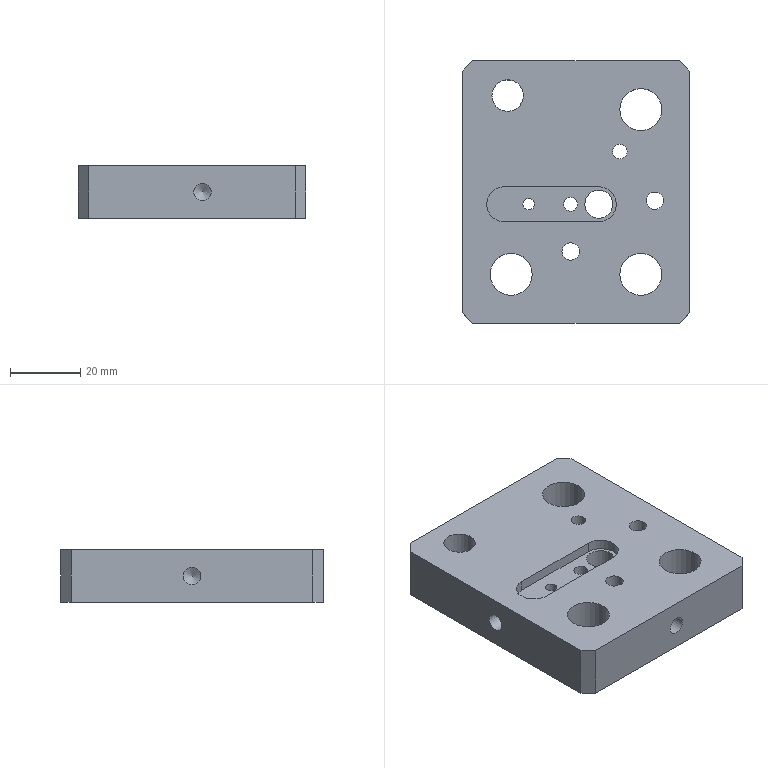Part | NX | features BREP 1 | 1 solid | 29 faces | box 65 x 75 x 15 mm | volume 63504 mm3 | cylinder 14 | plane 13 | cone 2 | commonest cylinder face diameters 5 x4 12 x3 10 x2 3.3 x1 4 x1 4.2 x1
STEP:
#1=CARTESIAN_POINT('',(32.5,-34.5,0.));
#2=VERTEX_POINT('',#1);
#3=CARTESIAN_POINT('',(32.5,34.5,0.));
#4=VERTEX_POINT('',#3);
#5=CARTESIAN_POINT('',(32.5,37.5,0.));
#6=DIRECTION('',(0.,1.,0.));
#7=VECTOR('',#6,1000.);
#8=LINE('',#5,#7);
#9=EDGE_CURVE('',#2,#4,#8,.T.);
#10=ORIENTED_EDGE('',*,*,#9,.F.);
#11=CARTESIAN_POINT('',(32.5,-34.5,-15.));
#12=VERTEX_POINT('',#11);
#13=CARTESIAN_POINT('',(32.5,-34.5,-15.));
#14=DIRECTION('',(0.,0.,1.));
#15=VECTOR('',#14,1000.);
#16=LINE('',#13,#15);
#17=EDGE_CURVE('',#12,#2,#16,.T.);
#18=ORIENTED_EDGE('',*,*,#17,.F.);
#19=CARTESIAN_POINT('',(32.5,34.5,-15.));
#20=VERTEX_POINT('',#19);
#21=CARTESIAN_POINT('',(32.5,37.5,-15.));
#22=DIRECTION('',(0.,1.,0.));
#23=VECTOR('',#22,1000.);
#24=LINE('',#21,#23);
#25=EDGE_CURVE('',#12,#20,#24,.T.);
#26=ORIENTED_EDGE('',*,*,#25,.T.);
#27=CARTESIAN_POINT('',(32.5,34.5,-15.));
#28=DIRECTION('',(0.,0.,-1.));
#29=VECTOR('',#28,1000.);
#30=LINE('',#27,#29);
#31=EDGE_CURVE('',#4,#20,#30,.T.);
#32=ORIENTED_EDGE('',*,*,#31,.F.);
#33=EDGE_LOOP('',(#10,#18,#26,#32));
#34=FACE_BOUND('',#33,.T.);
#35=CARTESIAN_POINT('',(32.5,37.5,-15.));
#36=DIRECTION('',(-1.,0.,0.));
#37=DIRECTION('',(0.,1.,0.));
#38=AXIS2_PLACEMENT_3D('',#35,#36,#37);
#39=PLANE('',#38);
#40=ADVANCED_FACE('',(#34),#39,.F.);
#41=CARTESIAN_POINT('',(29.5,37.5,-15.));
#42=VERTEX_POINT('',#41);
#43=CARTESIAN_POINT('',(-29.5,37.5,-15.));
#44=VERTEX_POINT('',#43);
#45=CARTESIAN_POINT('',(-32.5,37.5,-15.));
#46=DIRECTION('',(-1.,0.,0.));
#47=VECTOR('',#46,1000.);
#48=LINE('',#45,#47);
#49=EDGE_CURVE('',#42,#44,#48,.T.);
#50=ORIENTED_EDGE('',*,*,#49,.T.);
#51=CARTESIAN_POINT('',(-29.5,37.5,0.));
#52=VERTEX_POINT('',#51);
#53=CARTESIAN_POINT('',(-29.5,37.5,-15.));
#54=DIRECTION('',(0.,0.,-1.));
#55=VECTOR('',#54,1000.);
#56=LINE('',#53,#55);
#57=EDGE_CURVE('',#52,#44,#56,.T.);
#58=ORIENTED_EDGE('',*,*,#57,.F.);
#59=CARTESIAN_POINT('',(29.5,37.5,0.));
#60=VERTEX_POINT('',#59);
#61=CARTESIAN_POINT('',(-32.5,37.5,0.));
#62=DIRECTION('',(-1.,0.,0.));
#63=VECTOR('',#62,1000.);
#64=LINE('',#61,#63);
#65=EDGE_CURVE('',#60,#52,#64,.T.);
#66=ORIENTED_EDGE('',*,*,#65,.F.);
#67=CARTESIAN_POINT('',(29.5,37.5,-15.));
#68=DIRECTION('',(0.,0.,1.));
#69=VECTOR('',#68,1000.);
#70=LINE('',#67,#69);
#71=EDGE_CURVE('',#42,#60,#70,.T.);
#72=ORIENTED_EDGE('',*,*,#71,.F.);
#73=EDGE_LOOP('',(#50,#58,#66,#72));
#74=FACE_BOUND('',#73,.T.);
#75=CARTESIAN_POINT('',(-32.5,37.5,-15.));
#76=DIRECTION('',(0.,-1.,0.));
#77=DIRECTION('',(0.,0.,-1.));
#78=AXIS2_PLACEMENT_3D('',#75,#76,#77);
#79=PLANE('',#78);
#80=ADVANCED_FACE('',(#74),#79,.F.);
#81=CARTESIAN_POINT('',(-32.5,0.,-10.));
#82=VERTEX_POINT('',#81);
#83=CARTESIAN_POINT('',(-32.5,0.,-7.5));
#84=DIRECTION('',(1.,0.,0.));
#85=DIRECTION('',(0.,0.,-1.));
#86=AXIS2_PLACEMENT_3D('',#83,#84,#85);
#87=CIRCLE('',#86,2.5);
#88=EDGE_CURVE('',#82,#82,#87,.T.);
#89=ORIENTED_EDGE('',*,*,#88,.T.);
#90=EDGE_LOOP('',(#89));
#91=FACE_BOUND('',#90,.T.);
#92=CARTESIAN_POINT('',(-32.5,34.5,-15.));
#93=VERTEX_POINT('',#92);
#94=CARTESIAN_POINT('',(-32.5,-34.5,-15.));
#95=VERTEX_POINT('',#94);
#96=CARTESIAN_POINT('',(-32.5,37.5,-15.));
#97=DIRECTION('',(0.,-1.,0.));
#98=VECTOR('',#97,1000.);
#99=LINE('',#96,#98);
#100=EDGE_CURVE('',#93,#95,#99,.T.);
#101=ORIENTED_EDGE('',*,*,#100,.T.);
#102=CARTESIAN_POINT('',(-32.5,-34.5,0.));
#103=VERTEX_POINT('',#102);
#104=CARTESIAN_POINT('',(-32.5,-34.5,-15.));
#105=DIRECTION('',(0.,0.,-1.));
#106=VECTOR('',#105,1000.);
#107=LINE('',#104,#106);
#108=EDGE_CURVE('',#103,#95,#107,.T.);
#109=ORIENTED_EDGE('',*,*,#108,.F.);
#110=CARTESIAN_POINT('',(-32.5,34.5,0.));
#111=VERTEX_POINT('',#110);
#112=CARTESIAN_POINT('',(-32.5,37.5,0.));
#113=DIRECTION('',(0.,-1.,0.));
#114=VECTOR('',#113,1000.);
#115=LINE('',#112,#114);
#116=EDGE_CURVE('',#111,#103,#115,.T.);
#117=ORIENTED_EDGE('',*,*,#116,.F.);
#118=CARTESIAN_POINT('',(-32.5,34.5,-15.));
#119=DIRECTION('',(0.,0.,1.));
#120=VECTOR('',#119,1000.);
#121=LINE('',#118,#120);
#122=EDGE_CURVE('',#93,#111,#121,.T.);
#123=ORIENTED_EDGE('',*,*,#122,.F.);
#124=EDGE_LOOP('',(#101,#109,#117,#123));
#125=FACE_BOUND('',#124,.T.);
#126=CARTESIAN_POINT('',(-32.5,37.5,-15.));
#127=DIRECTION('',(1.,0.,0.));
#128=DIRECTION('',(0.,-1.,0.));
#129=AXIS2_PLACEMENT_3D('',#126,#127,#128);
#130=PLANE('',#129);
#131=ADVANCED_FACE('',(#91,#125),#130,.F.);
#132=CARTESIAN_POINT('',(3.,-37.5,-5.));
#133=VERTEX_POINT('',#132);
#134=CARTESIAN_POINT('',(3.,-37.5,-7.5));
#135=DIRECTION('',(0.,1.,0.));
#136=DIRECTION('',(0.,0.,1.));
#137=AXIS2_PLACEMENT_3D('',#134,#135,#136);
#138=CIRCLE('',#137,2.5);
#139=EDGE_CURVE('',#133,#133,#138,.T.);
#140=ORIENTED_EDGE('',*,*,#139,.T.);
#141=EDGE_LOOP('',(#140));
#142=FACE_BOUND('',#141,.T.);
#143=CARTESIAN_POINT('',(-29.5,-37.5,0.));
#144=VERTEX_POINT('',#143);
#145=CARTESIAN_POINT('',(29.5,-37.5,0.));
#146=VERTEX_POINT('',#145);
#147=CARTESIAN_POINT('',(-32.5,-37.5,0.));
#148=DIRECTION('',(1.,0.,0.));
#149=VECTOR('',#148,1000.);
#150=LINE('',#147,#149);
#151=EDGE_CURVE('',#144,#146,#150,.T.);
#152=ORIENTED_EDGE('',*,*,#151,.F.);
#153=CARTESIAN_POINT('',(-29.5,-37.5,-15.));
#154=VERTEX_POINT('',#153);
#155=CARTESIAN_POINT('',(-29.5,-37.5,-15.));
#156=DIRECTION('',(0.,0.,1.));
#157=VECTOR('',#156,1000.);
#158=LINE('',#155,#157);
#159=EDGE_CURVE('',#154,#144,#158,.T.);
#160=ORIENTED_EDGE('',*,*,#159,.F.);
#161=CARTESIAN_POINT('',(29.5,-37.5,-15.));
#162=VERTEX_POINT('',#161);
#163=CARTESIAN_POINT('',(-32.5,-37.5,-15.));
#164=DIRECTION('',(1.,0.,0.));
#165=VECTOR('',#164,1000.);
#166=LINE('',#163,#165);
#167=EDGE_CURVE('',#154,#162,#166,.T.);
#168=ORIENTED_EDGE('',*,*,#167,.T.);
#169=CARTESIAN_POINT('',(29.5,-37.5,-15.));
#170=DIRECTION('',(0.,0.,-1.));
#171=VECTOR('',#170,1000.);
#172=LINE('',#169,#171);
#173=EDGE_CURVE('',#146,#162,#172,.T.);
#174=ORIENTED_EDGE('',*,*,#173,.F.);
#175=EDGE_LOOP('',(#152,#160,#168,#174));
#176=FACE_BOUND('',#175,.T.);
#177=CARTESIAN_POINT('',(-32.5,-37.5,-15.));
#178=DIRECTION('',(0.,1.,0.));
#179=DIRECTION('',(0.,0.,1.));
#180=AXIS2_PLACEMENT_3D('',#177,#178,#179);
#181=PLANE('',#180);
#182=ADVANCED_FACE('',(#142,#176),#181,.F.);
#183=CARTESIAN_POINT('',(10.4,11.5,-15.));
#184=VERTEX_POINT('',#183);
#185=CARTESIAN_POINT('',(12.5,11.5,-15.));
#186=DIRECTION('',(0.,0.,-1.));
#187=DIRECTION('',(-1.,0.,0.));
#188=AXIS2_PLACEMENT_3D('',#185,#186,#187);
#189=CIRCLE('',#188,2.1);
#190=EDGE_CURVE('',#184,#184,#189,.T.);
#191=ORIENTED_EDGE('',*,*,#190,.F.);
#192=EDGE_LOOP('',(#191));
#193=FACE_BOUND('',#192,.T.);
#194=CARTESIAN_POINT('',(-3.5,-3.5,-15.));
#195=VERTEX_POINT('',#194);
#196=CARTESIAN_POINT('',(-1.5,-3.5,-15.));
#197=DIRECTION('',(0.,0.,-1.));
#198=DIRECTION('',(-1.,0.,0.));
#199=AXIS2_PLACEMENT_3D('',#196,#197,#198);
#200=CIRCLE('',#199,2.);
#201=EDGE_CURVE('',#195,#195,#200,.T.);
#202=ORIENTED_EDGE('',*,*,#201,.F.);
#203=EDGE_LOOP('',(#202));
#204=FACE_BOUND('',#203,.T.);
#205=CARTESIAN_POINT('',(-15.15,-3.5,-15.));
#206=VERTEX_POINT('',#205);
#207=CARTESIAN_POINT('',(-13.5,-3.5,-15.));
#208=DIRECTION('',(0.,0.,-1.));
#209=DIRECTION('',(-1.,0.,0.));
#210=AXIS2_PLACEMENT_3D('',#207,#208,#209);
#211=CIRCLE('',#210,1.65);
#212=EDGE_CURVE('',#206,#206,#211,.T.);
#213=ORIENTED_EDGE('',*,*,#212,.F.);
#214=EDGE_LOOP('',(#213));
#215=FACE_BOUND('',#214,.T.);
#216=CARTESIAN_POINT('',(2.5,-3.5,-15.));
#217=VERTEX_POINT('',#216);
#218=CARTESIAN_POINT('',(6.5,-3.5,-15.));
#219=DIRECTION('',(0.,0.,-1.));
#220=DIRECTION('',(-1.,0.,0.));
#221=AXIS2_PLACEMENT_3D('',#218,#219,#220);
#222=CIRCLE('',#221,4.);
#223=EDGE_CURVE('',#217,#217,#222,.T.);
#224=ORIENTED_EDGE('',*,*,#223,.F.);
#225=EDGE_LOOP('',(#224));
#226=FACE_BOUND('',#225,.T.);
#227=CARTESIAN_POINT('',(-24.,27.5,-15.));
#228=VERTEX_POINT('',#227);
#229=CARTESIAN_POINT('',(-19.5,27.5,-15.));
#230=DIRECTION('',(0.,0.,-1.));
#231=DIRECTION('',(-1.,0.,0.));
#232=AXIS2_PLACEMENT_3D('',#229,#230,#231);
#233=CIRCLE('',#232,4.5);
#234=EDGE_CURVE('',#228,#228,#233,.T.);
#235=ORIENTED_EDGE('',*,*,#234,.F.);
#236=EDGE_LOOP('',(#235));
#237=FACE_BOUND('',#236,.T.);
#238=CARTESIAN_POINT('',(20.,-2.5,-15.));
#239=VERTEX_POINT('',#238);
#240=CARTESIAN_POINT('',(22.5,-2.5,-15.));
#241=DIRECTION('',(0.,0.,-1.));
#242=DIRECTION('',(-1.,0.,0.));
#243=AXIS2_PLACEMENT_3D('',#240,#241,#242);
#244=CIRCLE('',#243,2.5);
#245=EDGE_CURVE('',#239,#239,#244,.T.);
#246=ORIENTED_EDGE('',*,*,#245,.F.);
#247=EDGE_LOOP('',(#246));
#248=FACE_BOUND('',#247,.T.);
#249=CARTESIAN_POINT('',(-4.,-17.,-15.));
#250=VERTEX_POINT('',#249);
#251=CARTESIAN_POINT('',(-1.5,-17.,-15.));
#252=DIRECTION('',(0.,0.,-1.));
#253=DIRECTION('',(-1.,0.,0.));
#254=AXIS2_PLACEMENT_3D('',#251,#252,#253);
#255=CIRCLE('',#254,2.5);
#256=EDGE_CURVE('',#250,#250,#255,.T.);
#257=ORIENTED_EDGE('',*,*,#256,.F.);
#258=EDGE_LOOP('',(#257));
#259=FACE_BOUND('',#258,.T.);
#260=CARTESIAN_POINT('',(12.5,-23.5,-15.));
#261=VERTEX_POINT('',#260);
#262=CARTESIAN_POINT('',(18.5,-23.5,-15.));
#263=DIRECTION('',(0.,0.,-1.));
#264=DIRECTION('',(-1.,0.,0.));
#265=AXIS2_PLACEMENT_3D('',#262,#263,#264);
#266=CIRCLE('',#265,6.);
#267=EDGE_CURVE('',#261,#261,#266,.T.);
#268=ORIENTED_EDGE('',*,*,#267,.F.);
#269=EDGE_LOOP('',(#268));
#270=FACE_BOUND('',#269,.T.);
#271=CARTESIAN_POINT('',(-24.5,-23.5,-15.));
#272=VERTEX_POINT('',#271);
#273=CARTESIAN_POINT('',(-18.5,-23.5,-15.));
#274=DIRECTION('',(0.,0.,-1.));
#275=DIRECTION('',(-1.,0.,0.));
#276=AXIS2_PLACEMENT_3D('',#273,#274,#275);
#277=CIRCLE('',#276,6.);
#278=EDGE_CURVE('',#272,#272,#277,.T.);
#279=ORIENTED_EDGE('',*,*,#278,.F.);
#280=EDGE_LOOP('',(#279));
#281=FACE_BOUND('',#280,.T.);
#282=CARTESIAN_POINT('',(12.5,23.5,-15.));
#283=VERTEX_POINT('',#282);
#284=CARTESIAN_POINT('',(18.5,23.5,-15.));
#285=DIRECTION('',(0.,0.,-1.));
#286=DIRECTION('',(-1.,0.,0.));
#287=AXIS2_PLACEMENT_3D('',#284,#285,#286);
#288=CIRCLE('',#287,6.);
#289=EDGE_CURVE('',#283,#283,#288,.T.);
#290=ORIENTED_EDGE('',*,*,#289,.F.);
#291=EDGE_LOOP('',(#290));
#292=FACE_BOUND('',#291,.T.);
#293=ORIENTED_EDGE('',*,*,#25,.F.);
#294=CARTESIAN_POINT('',(33.5,-33.5,-15.));
#295=DIRECTION('',(0.7071,0.7071,0.));
#296=VECTOR('',#295,1000.);
#297=LINE('',#294,#296);
#298=EDGE_CURVE('',#162,#12,#297,.T.);
#299=ORIENTED_EDGE('',*,*,#298,.F.);
#300=ORIENTED_EDGE('',*,*,#167,.F.);
#301=CARTESIAN_POINT('',(-33.5,-33.5,-15.));
#302=DIRECTION('',(0.7071,-0.7071,0.));
#303=VECTOR('',#302,1000.);
#304=LINE('',#301,#303);
#305=EDGE_CURVE('',#95,#154,#304,.T.);
#306=ORIENTED_EDGE('',*,*,#305,.F.);
#307=ORIENTED_EDGE('',*,*,#100,.F.);
#308=CARTESIAN_POINT('',(-33.5,33.5,-15.));
#309=DIRECTION('',(-0.7071,-0.7071,0.));
#310=VECTOR('',#309,1000.);
#311=LINE('',#308,#310);
#312=EDGE_CURVE('',#44,#93,#311,.T.);
#313=ORIENTED_EDGE('',*,*,#312,.F.);
#314=ORIENTED_EDGE('',*,*,#49,.F.);
#315=CARTESIAN_POINT('',(33.5,33.5,-15.));
#316=DIRECTION('',(-0.7071,0.7071,0.));
#317=VECTOR('',#316,1000.);
#318=LINE('',#315,#317);
#319=EDGE_CURVE('',#20,#42,#318,.T.);
#320=ORIENTED_EDGE('',*,*,#319,.F.);
#321=EDGE_LOOP('',(#293,#299,#300,#306,#307,#313,#314,#320));
#322=FACE_BOUND('',#321,.T.);
#323=CARTESIAN_POINT('',(0.,0.,-15.));
#324=DIRECTION('',(0.,0.,-1.));
#325=DIRECTION('',(-1.,0.,0.));
#326=AXIS2_PLACEMENT_3D('',#323,#324,#325);
#327=PLANE('',#326);
#328=ADVANCED_FACE('',(#193,#204,#215,#226,#237,#248,#259,#270,#281,#292,#322),#327,.T.);
#329=CARTESIAN_POINT('',(10.4,11.5,0.));
#330=VERTEX_POINT('',#329);
#331=CARTESIAN_POINT('',(12.5,11.5,0.));
#332=DIRECTION('',(0.,0.,-1.));
#333=DIRECTION('',(-1.,0.,0.));
#334=AXIS2_PLACEMENT_3D('',#331,#332,#333);
#335=CIRCLE('',#334,2.1);
#336=EDGE_CURVE('',#330,#330,#335,.T.);
#337=ORIENTED_EDGE('',*,*,#336,.T.);
#338=EDGE_LOOP('',(#337));
#339=FACE_BOUND('',#338,.T.);
#340=CARTESIAN_POINT('',(-24.,27.5,0.));
#341=VERTEX_POINT('',#340);
#342=CARTESIAN_POINT('',(-19.5,27.5,0.));
#343=DIRECTION('',(0.,0.,-1.));
#344=DIRECTION('',(-1.,0.,0.));
#345=AXIS2_PLACEMENT_3D('',#342,#343,#344);
#346=CIRCLE('',#345,4.5);
#347=EDGE_CURVE('',#341,#341,#346,.T.);
#348=ORIENTED_EDGE('',*,*,#347,.T.);
#349=EDGE_LOOP('',(#348));
#350=FACE_BOUND('',#349,.T.);
#351=CARTESIAN_POINT('',(20.,-2.5,0.));
#352=VERTEX_POINT('',#351);
#353=CARTESIAN_POINT('',(22.5,-2.5,0.));
#354=DIRECTION('',(0.,0.,-1.));
#355=DIRECTION('',(-1.,0.,0.));
#356=AXIS2_PLACEMENT_3D('',#353,#354,#355);
#357=CIRCLE('',#356,2.5);
#358=EDGE_CURVE('',#352,#352,#357,.T.);
#359=ORIENTED_EDGE('',*,*,#358,.T.);
#360=EDGE_LOOP('',(#359));
#361=FACE_BOUND('',#360,.T.);
#362=CARTESIAN_POINT('',(-4.,-17.,0.));
#363=VERTEX_POINT('',#362);
#364=CARTESIAN_POINT('',(-1.5,-17.,0.));
#365=DIRECTION('',(0.,0.,-1.));
#366=DIRECTION('',(-1.,0.,0.));
#367=AXIS2_PLACEMENT_3D('',#364,#365,#366);
#368=CIRCLE('',#367,2.5);
#369=EDGE_CURVE('',#363,#363,#368,.T.);
#370=ORIENTED_EDGE('',*,*,#369,.T.);
#371=EDGE_LOOP('',(#370));
#372=FACE_BOUND('',#371,.T.);
#373=CARTESIAN_POINT('',(12.5,-23.5,0.));
#374=VERTEX_POINT('',#373);
#375=CARTESIAN_POINT('',(18.5,-23.5,0.));
#376=DIRECTION('',(0.,0.,-1.));
#377=DIRECTION('',(-1.,0.,0.));
#378=AXIS2_PLACEMENT_3D('',#375,#376,#377);
#379=CIRCLE('',#378,6.);
#380=EDGE_CURVE('',#374,#374,#379,.T.);
#381=ORIENTED_EDGE('',*,*,#380,.T.);
#382=EDGE_LOOP('',(#381));
#383=FACE_BOUND('',#382,.T.);
#384=CARTESIAN_POINT('',(-24.5,-23.5,0.));
#385=VERTEX_POINT('',#384);
#386=CARTESIAN_POINT('',(-18.5,-23.5,0.));
#387=DIRECTION('',(0.,0.,-1.));
#388=DIRECTION('',(-1.,0.,0.));
#389=AXIS2_PLACEMENT_3D('',#386,#387,#388);
#390=CIRCLE('',#389,6.);
#391=EDGE_CURVE('',#385,#385,#390,.T.);
#392=ORIENTED_EDGE('',*,*,#391,.T.);
#393=EDGE_LOOP('',(#392));
#394=FACE_BOUND('',#393,.T.);
#395=CARTESIAN_POINT('',(12.5,23.5,0.));
#396=VERTEX_POINT('',#395);
#397=CARTESIAN_POINT('',(18.5,23.5,0.));
#398=DIRECTION('',(0.,0.,-1.));
#399=DIRECTION('',(-1.,0.,0.));
#400=AXIS2_PLACEMENT_3D('',#397,#398,#399);
#401=CIRCLE('',#400,6.);
#402=EDGE_CURVE('',#396,#396,#401,.T.);
#403=ORIENTED_EDGE('',*,*,#402,.T.);
#404=EDGE_LOOP('',(#403));
#405=FACE_BOUND('',#404,.T.);
#406=CARTESIAN_POINT('',(6.5,-8.5,0.));
#407=VERTEX_POINT('',#406);
#408=CARTESIAN_POINT('',(-20.5,-8.5,0.));
#409=VERTEX_POINT('',#408);
#410=CARTESIAN_POINT('',(6.5,-8.5,0.));
#411=DIRECTION('',(-1.,0.,0.));
#412=VECTOR('',#411,1000.);
#413=LINE('',#410,#412);
#414=EDGE_CURVE('',#407,#409,#413,.T.);
#415=ORIENTED_EDGE('',*,*,#414,.T.);
#416=CARTESIAN_POINT('',(-20.5,1.5,0.));
#417=VERTEX_POINT('',#416);
#418=CARTESIAN_POINT('',(-20.5,-3.5,0.));
#419=DIRECTION('',(0.,0.,-1.));
#420=DIRECTION('',(-1.,0.,0.));
#421=AXIS2_PLACEMENT_3D('',#418,#419,#420);
#422=CIRCLE('',#421,5.);
#423=EDGE_CURVE('',#409,#417,#422,.T.);
#424=ORIENTED_EDGE('',*,*,#423,.T.);
#425=CARTESIAN_POINT('',(6.5,1.5,0.));
#426=VERTEX_POINT('',#425);
#427=CARTESIAN_POINT('',(6.5,1.5,0.));
#428=DIRECTION('',(1.,0.,0.));
#429=VECTOR('',#428,1000.);
#430=LINE('',#427,#429);
#431=EDGE_CURVE('',#417,#426,#430,.T.);
#432=ORIENTED_EDGE('',*,*,#431,.T.);
#433=CARTESIAN_POINT('',(6.5,-3.5,0.));
#434=DIRECTION('',(0.,0.,-1.));
#435=DIRECTION('',(-1.,0.,0.));
#436=AXIS2_PLACEMENT_3D('',#433,#434,#435);
#437=CIRCLE('',#436,5.);
#438=EDGE_CURVE('',#426,#407,#437,.T.);
#439=ORIENTED_EDGE('',*,*,#438,.T.);
#440=EDGE_LOOP('',(#415,#424,#432,#439));
#441=FACE_BOUND('',#440,.T.);
#442=ORIENTED_EDGE('',*,*,#65,.T.);
#443=CARTESIAN_POINT('',(-32.5,34.5,0.));
#444=DIRECTION('',(0.7071,0.7071,0.));
#445=VECTOR('',#444,1000.);
#446=LINE('',#443,#445);
#447=EDGE_CURVE('',#111,#52,#446,.T.);
#448=ORIENTED_EDGE('',*,*,#447,.F.);
#449=ORIENTED_EDGE('',*,*,#116,.T.);
#450=CARTESIAN_POINT('',(-29.5,-37.5,0.));
#451=DIRECTION('',(-0.7071,0.7071,0.));
#452=VECTOR('',#451,1000.);
#453=LINE('',#450,#452);
#454=EDGE_CURVE('',#144,#103,#453,.T.);
#455=ORIENTED_EDGE('',*,*,#454,.F.);
#456=ORIENTED_EDGE('',*,*,#151,.T.);
#457=CARTESIAN_POINT('',(32.5,-34.5,0.));
#458=DIRECTION('',(-0.7071,-0.7071,0.));
#459=VECTOR('',#458,1000.);
#460=LINE('',#457,#459);
#461=EDGE_CURVE('',#2,#146,#460,.T.);
#462=ORIENTED_EDGE('',*,*,#461,.F.);
#463=ORIENTED_EDGE('',*,*,#9,.T.);
#464=CARTESIAN_POINT('',(29.5,37.5,0.));
#465=DIRECTION('',(0.7071,-0.7071,0.));
#466=VECTOR('',#465,1000.);
#467=LINE('',#464,#466);
#468=EDGE_CURVE('',#60,#4,#467,.T.);
#469=ORIENTED_EDGE('',*,*,#468,.F.);
#470=EDGE_LOOP('',(#442,#448,#449,#455,#456,#462,#463,#469));
#471=FACE_BOUND('',#470,.T.);
#472=CARTESIAN_POINT('',(0.,0.,0.));
#473=DIRECTION('',(0.,0.,-1.));
#474=DIRECTION('',(-1.,0.,0.));
#475=AXIS2_PLACEMENT_3D('',#472,#473,#474);
#476=PLANE('',#475);
#477=ADVANCED_FACE('',(#339,#350,#361,#372,#383,#394,#405,#441,#471),#476,.F.);
#478=ORIENTED_EDGE('',*,*,#438,.F.);
#479=CARTESIAN_POINT('',(6.5,1.5,-3.));
#480=VERTEX_POINT('',#479);
#481=CARTESIAN_POINT('',(6.5,1.5,-3.));
#482=DIRECTION('',(0.,0.,1.));
#483=VECTOR('',#482,1000.);
#484=LINE('',#481,#483);
#485=EDGE_CURVE('',#480,#426,#484,.T.);
#486=ORIENTED_EDGE('',*,*,#485,.F.);
#487=CARTESIAN_POINT('',(6.5,-8.5,-3.));
#488=VERTEX_POINT('',#487);
#489=CARTESIAN_POINT('',(6.5,-3.5,-3.));
#490=DIRECTION('',(0.,0.,-1.));
#491=DIRECTION('',(-1.,0.,0.));
#492=AXIS2_PLACEMENT_3D('',#489,#490,#491);
#493=CIRCLE('',#492,5.);
#494=EDGE_CURVE('',#480,#488,#493,.T.);
#495=ORIENTED_EDGE('',*,*,#494,.T.);
#496=CARTESIAN_POINT('',(6.5,-8.5,-3.));
#497=DIRECTION('',(0.,0.,1.));
#498=VECTOR('',#497,1000.);
#499=LINE('',#496,#498);
#500=EDGE_CURVE('',#488,#407,#499,.T.);
#501=ORIENTED_EDGE('',*,*,#500,.T.);
#502=EDGE_LOOP('',(#478,#486,#495,#501));
#503=FACE_BOUND('',#502,.T.);
#504=CARTESIAN_POINT('',(6.5,-3.5,-3.));
#505=DIRECTION('',(0.,0.,1.));
#506=DIRECTION('',(1.,0.,0.));
#507=AXIS2_PLACEMENT_3D('',#504,#505,#506);
#508=CYLINDRICAL_SURFACE('',#507,5.);
#509=ADVANCED_FACE('',(#503),#508,.F.);
#510=ORIENTED_EDGE('',*,*,#431,.F.);
#511=CARTESIAN_POINT('',(-20.5,1.5,-3.));
#512=VERTEX_POINT('',#511);
#513=CARTESIAN_POINT('',(-20.5,1.5,-3.));
#514=DIRECTION('',(0.,0.,1.));
#515=VECTOR('',#514,1000.);
#516=LINE('',#513,#515);
#517=EDGE_CURVE('',#512,#417,#516,.T.);
#518=ORIENTED_EDGE('',*,*,#517,.F.);
#519=CARTESIAN_POINT('',(6.5,1.5,-3.));
#520=DIRECTION('',(1.,0.,0.));
#521=VECTOR('',#520,1000.);
#522=LINE('',#519,#521);
#523=EDGE_CURVE('',#512,#480,#522,.T.);
#524=ORIENTED_EDGE('',*,*,#523,.T.);
#525=ORIENTED_EDGE('',*,*,#485,.T.);
#526=EDGE_LOOP('',(#510,#518,#524,#525));
#527=FACE_BOUND('',#526,.T.);
#528=CARTESIAN_POINT('',(6.5,1.5,-3.));
#529=DIRECTION('',(0.,1.,0.));
#530=DIRECTION('',(0.,0.,1.));
#531=AXIS2_PLACEMENT_3D('',#528,#529,#530);
#532=PLANE('',#531);
#533=ADVANCED_FACE('',(#527),#532,.F.);
#534=ORIENTED_EDGE('',*,*,#423,.F.);
#535=CARTESIAN_POINT('',(-20.5,-8.5,-3.));
#536=VERTEX_POINT('',#535);
#537=CARTESIAN_POINT('',(-20.5,-8.5,-3.));
#538=DIRECTION('',(0.,0.,1.));
#539=VECTOR('',#538,1000.);
#540=LINE('',#537,#539);
#541=EDGE_CURVE('',#536,#409,#540,.T.);
#542=ORIENTED_EDGE('',*,*,#541,.F.);
#543=CARTESIAN_POINT('',(-20.5,-3.5,-3.));
#544=DIRECTION('',(0.,0.,-1.));
#545=DIRECTION('',(-1.,0.,0.));
#546=AXIS2_PLACEMENT_3D('',#543,#544,#545);
#547=CIRCLE('',#546,5.);
#548=EDGE_CURVE('',#536,#512,#547,.T.);
#549=ORIENTED_EDGE('',*,*,#548,.T.);
#550=ORIENTED_EDGE('',*,*,#517,.T.);
#551=EDGE_LOOP('',(#534,#542,#549,#550));
#552=FACE_BOUND('',#551,.T.);
#553=CARTESIAN_POINT('',(-20.5,-3.5,-3.));
#554=DIRECTION('',(0.,0.,1.));
#555=DIRECTION('',(1.,0.,0.));
#556=AXIS2_PLACEMENT_3D('',#553,#554,#555);
#557=CYLINDRICAL_SURFACE('',#556,5.);
#558=ADVANCED_FACE('',(#552),#557,.F.);
#559=ORIENTED_EDGE('',*,*,#414,.F.);
#560=ORIENTED_EDGE('',*,*,#500,.F.);
#561=CARTESIAN_POINT('',(6.5,-8.5,-3.));
#562=DIRECTION('',(-1.,0.,0.));
#563=VECTOR('',#562,1000.);
#564=LINE('',#561,#563);
#565=EDGE_CURVE('',#488,#536,#564,.T.);
#566=ORIENTED_EDGE('',*,*,#565,.T.);
#567=ORIENTED_EDGE('',*,*,#541,.T.);
#568=EDGE_LOOP('',(#559,#560,#566,#567));
#569=FACE_BOUND('',#568,.T.);
#570=CARTESIAN_POINT('',(6.5,-8.5,-3.));
#571=DIRECTION('',(0.,-1.,0.));
#572=DIRECTION('',(0.,0.,-1.));
#573=AXIS2_PLACEMENT_3D('',#570,#571,#572);
#574=PLANE('',#573);
#575=ADVANCED_FACE('',(#569),#574,.F.);
#576=CARTESIAN_POINT('',(-3.5,-3.5,-3.));
#577=VERTEX_POINT('',#576);
#578=CARTESIAN_POINT('',(-1.5,-3.5,-3.));
#579=DIRECTION('',(0.,0.,-1.));
#580=DIRECTION('',(-1.,0.,0.));
#581=AXIS2_PLACEMENT_3D('',#578,#579,#580);
#582=CIRCLE('',#581,2.);
#583=EDGE_CURVE('',#577,#577,#582,.T.);
#584=ORIENTED_EDGE('',*,*,#583,.T.);
#585=EDGE_LOOP('',(#584));
#586=FACE_BOUND('',#585,.T.);
#587=CARTESIAN_POINT('',(-15.15,-3.5,-3.));
#588=VERTEX_POINT('',#587);
#589=CARTESIAN_POINT('',(-13.5,-3.5,-3.));
#590=DIRECTION('',(0.,0.,-1.));
#591=DIRECTION('',(-1.,0.,0.));
#592=AXIS2_PLACEMENT_3D('',#589,#590,#591);
#593=CIRCLE('',#592,1.65);
#594=EDGE_CURVE('',#588,#588,#593,.T.);
#595=ORIENTED_EDGE('',*,*,#594,.T.);
#596=EDGE_LOOP('',(#595));
#597=FACE_BOUND('',#596,.T.);
#598=CARTESIAN_POINT('',(2.5,-3.5,-3.));
#599=VERTEX_POINT('',#598);
#600=CARTESIAN_POINT('',(6.5,-3.5,-3.));
#601=DIRECTION('',(0.,0.,-1.));
#602=DIRECTION('',(-1.,0.,0.));
#603=AXIS2_PLACEMENT_3D('',#600,#601,#602);
#604=CIRCLE('',#603,4.);
#605=EDGE_CURVE('',#599,#599,#604,.T.);
#606=ORIENTED_EDGE('',*,*,#605,.T.);
#607=EDGE_LOOP('',(#606));
#608=FACE_BOUND('',#607,.T.);
#609=ORIENTED_EDGE('',*,*,#494,.F.);
#610=ORIENTED_EDGE('',*,*,#523,.F.);
#611=ORIENTED_EDGE('',*,*,#548,.F.);
#612=ORIENTED_EDGE('',*,*,#565,.F.);
#613=EDGE_LOOP('',(#609,#610,#611,#612));
#614=FACE_BOUND('',#613,.T.);
#615=CARTESIAN_POINT('',(6.5,-3.5,-3.));
#616=DIRECTION('',(0.,0.,1.));
#617=DIRECTION('',(1.,0.,0.));
#618=AXIS2_PLACEMENT_3D('',#615,#616,#617);
#619=PLANE('',#618);
#620=ADVANCED_FACE('',(#586,#597,#608,#614),#619,.T.);
#621=ORIENTED_EDGE('',*,*,#289,.T.);
#622=EDGE_LOOP('',(#621));
#623=FACE_BOUND('',#622,.T.);
#624=ORIENTED_EDGE('',*,*,#402,.F.);
#625=EDGE_LOOP('',(#624));
#626=FACE_BOUND('',#625,.T.);
#627=CARTESIAN_POINT('',(18.5,23.5,0.));
#628=DIRECTION('',(0.,0.,1.));
#629=DIRECTION('',(1.,0.,0.));
#630=AXIS2_PLACEMENT_3D('',#627,#628,#629);
#631=CYLINDRICAL_SURFACE('',#630,6.);
#632=ADVANCED_FACE('',(#623,#626),#631,.F.);
#633=ORIENTED_EDGE('',*,*,#278,.T.);
#634=EDGE_LOOP('',(#633));
#635=FACE_BOUND('',#634,.T.);
#636=ORIENTED_EDGE('',*,*,#391,.F.);
#637=EDGE_LOOP('',(#636));
#638=FACE_BOUND('',#637,.T.);
#639=CARTESIAN_POINT('',(-18.5,-23.5,0.));
#640=DIRECTION('',(0.,0.,1.));
#641=DIRECTION('',(1.,0.,0.));
#642=AXIS2_PLACEMENT_3D('',#639,#640,#641);
#643=CYLINDRICAL_SURFACE('',#642,6.);
#644=ADVANCED_FACE('',(#635,#638),#643,.F.);
#645=ORIENTED_EDGE('',*,*,#267,.T.);
#646=EDGE_LOOP('',(#645));
#647=FACE_BOUND('',#646,.T.);
#648=ORIENTED_EDGE('',*,*,#380,.F.);
#649=EDGE_LOOP('',(#648));
#650=FACE_BOUND('',#649,.T.);
#651=CARTESIAN_POINT('',(18.5,-23.5,0.));
#652=DIRECTION('',(0.,0.,1.));
#653=DIRECTION('',(1.,0.,0.));
#654=AXIS2_PLACEMENT_3D('',#651,#652,#653);
#655=CYLINDRICAL_SURFACE('',#654,6.);
#656=ADVANCED_FACE('',(#647,#650),#655,.F.);
#657=ORIENTED_EDGE('',*,*,#256,.T.);
#658=EDGE_LOOP('',(#657));
#659=FACE_BOUND('',#658,.T.);
#660=ORIENTED_EDGE('',*,*,#369,.F.);
#661=EDGE_LOOP('',(#660));
#662=FACE_BOUND('',#661,.T.);
#663=CARTESIAN_POINT('',(-1.5,-17.,0.));
#664=DIRECTION('',(0.,0.,1.));
#665=DIRECTION('',(1.,0.,0.));
#666=AXIS2_PLACEMENT_3D('',#663,#664,#665);
#667=CYLINDRICAL_SURFACE('',#666,2.5);
#668=ADVANCED_FACE('',(#659,#662),#667,.F.);
#669=ORIENTED_EDGE('',*,*,#245,.T.);
#670=EDGE_LOOP('',(#669));
#671=FACE_BOUND('',#670,.T.);
#672=ORIENTED_EDGE('',*,*,#358,.F.);
#673=EDGE_LOOP('',(#672));
#674=FACE_BOUND('',#673,.T.);
#675=CARTESIAN_POINT('',(22.5,-2.5,0.));
#676=DIRECTION('',(0.,0.,1.));
#677=DIRECTION('',(1.,0.,0.));
#678=AXIS2_PLACEMENT_3D('',#675,#676,#677);
#679=CYLINDRICAL_SURFACE('',#678,2.5);
#680=ADVANCED_FACE('',(#671,#674),#679,.F.);
#681=CARTESIAN_POINT('',(3.,-20.998,-7.5));
#682=VERTEX_POINT('',#681);
#683=VERTEX_LOOP('',#682);
#684=FACE_BOUND('',#683,.T.);
#685=CARTESIAN_POINT('',(3.,-22.5,-5.));
#686=VERTEX_POINT('',#685);
#687=CARTESIAN_POINT('',(3.,-22.5,-7.5));
#688=DIRECTION('',(0.,1.,0.));
#689=DIRECTION('',(0.,0.,1.));
#690=AXIS2_PLACEMENT_3D('',#687,#688,#689);
#691=CIRCLE('',#690,2.5);
#692=EDGE_CURVE('',#686,#686,#691,.T.);
#693=ORIENTED_EDGE('',*,*,#692,.F.);
#694=EDGE_LOOP('',(#693));
#695=FACE_BOUND('',#694,.T.);
#696=CARTESIAN_POINT('',(3.,-22.5,-7.5));
#697=DIRECTION('',(0.,-1.,0.));
#698=DIRECTION('',(0.,0.,-1.));
#699=AXIS2_PLACEMENT_3D('',#696,#697,#698);
#700=CONICAL_SURFACE('',#699,2.5,1.03);
#701=ADVANCED_FACE('',(#684,#695),#700,.F.);
#702=ORIENTED_EDGE('',*,*,#692,.T.);
#703=EDGE_LOOP('',(#702));
#704=FACE_BOUND('',#703,.T.);
#705=ORIENTED_EDGE('',*,*,#139,.F.);
#706=EDGE_LOOP('',(#705));
#707=FACE_BOUND('',#706,.T.);
#708=CARTESIAN_POINT('',(3.,-37.5,-7.5));
#709=DIRECTION('',(0.,-1.,0.));
#710=DIRECTION('',(0.,0.,-1.));
#711=AXIS2_PLACEMENT_3D('',#708,#709,#710);
#712=CYLINDRICAL_SURFACE('',#711,2.5);
#713=ADVANCED_FACE('',(#704,#707),#712,.F.);
#714=CARTESIAN_POINT('',(-15.998,0.,-7.5));
#715=VERTEX_POINT('',#714);
#716=VERTEX_LOOP('',#715);
#717=FACE_BOUND('',#716,.T.);
#718=CARTESIAN_POINT('',(-17.5,0.,-10.));
#719=VERTEX_POINT('',#718);
#720=CARTESIAN_POINT('',(-17.5,0.,-7.5));
#721=DIRECTION('',(1.,0.,0.));
#722=DIRECTION('',(0.,0.,-1.));
#723=AXIS2_PLACEMENT_3D('',#720,#721,#722);
#724=CIRCLE('',#723,2.5);
#725=EDGE_CURVE('',#719,#719,#724,.T.);
#726=ORIENTED_EDGE('',*,*,#725,.F.);
#727=EDGE_LOOP('',(#726));
#728=FACE_BOUND('',#727,.T.);
#729=CARTESIAN_POINT('',(-17.5,0.,-7.5));
#730=DIRECTION('',(-1.,0.,0.));
#731=DIRECTION('',(0.,0.,1.));
#732=AXIS2_PLACEMENT_3D('',#729,#730,#731);
#733=CONICAL_SURFACE('',#732,2.5,1.03);
#734=ADVANCED_FACE('',(#717,#728),#733,.F.);
#735=ORIENTED_EDGE('',*,*,#725,.T.);
#736=EDGE_LOOP('',(#735));
#737=FACE_BOUND('',#736,.T.);
#738=ORIENTED_EDGE('',*,*,#88,.F.);
#739=EDGE_LOOP('',(#738));
#740=FACE_BOUND('',#739,.T.);
#741=CARTESIAN_POINT('',(-32.5,0.,-7.5));
#742=DIRECTION('',(-1.,0.,0.));
#743=DIRECTION('',(0.,0.,1.));
#744=AXIS2_PLACEMENT_3D('',#741,#742,#743);
#745=CYLINDRICAL_SURFACE('',#744,2.5);
#746=ADVANCED_FACE('',(#737,#740),#745,.F.);
#747=ORIENTED_EDGE('',*,*,#319,.T.);
#748=ORIENTED_EDGE('',*,*,#71,.T.);
#749=ORIENTED_EDGE('',*,*,#468,.T.);
#750=ORIENTED_EDGE('',*,*,#31,.T.);
#751=EDGE_LOOP('',(#747,#748,#749,#750));
#752=FACE_BOUND('',#751,.T.);
#753=CARTESIAN_POINT('',(29.5,37.5,-15.));
#754=DIRECTION('',(-0.7071,-0.7071,0.));
#755=DIRECTION('',(0.,0.,-1.));
#756=AXIS2_PLACEMENT_3D('',#753,#754,#755);
#757=PLANE('',#756);
#758=ADVANCED_FACE('',(#752),#757,.F.);
#759=ORIENTED_EDGE('',*,*,#312,.T.);
#760=ORIENTED_EDGE('',*,*,#122,.T.);
#761=ORIENTED_EDGE('',*,*,#447,.T.);
#762=ORIENTED_EDGE('',*,*,#57,.T.);
#763=EDGE_LOOP('',(#759,#760,#761,#762));
#764=FACE_BOUND('',#763,.T.);
#765=CARTESIAN_POINT('',(-32.5,34.5,-15.));
#766=DIRECTION('',(0.7071,-0.7071,0.));
#767=DIRECTION('',(0.,0.,-1.));
#768=AXIS2_PLACEMENT_3D('',#765,#766,#767);
#769=PLANE('',#768);
#770=ADVANCED_FACE('',(#764),#769,.F.);
#771=ORIENTED_EDGE('',*,*,#298,.T.);
#772=ORIENTED_EDGE('',*,*,#17,.T.);
#773=ORIENTED_EDGE('',*,*,#461,.T.);
#774=ORIENTED_EDGE('',*,*,#173,.T.);
#775=EDGE_LOOP('',(#771,#772,#773,#774));
#776=FACE_BOUND('',#775,.T.);
#777=CARTESIAN_POINT('',(32.5,-34.5,-15.));
#778=DIRECTION('',(-0.7071,0.7071,0.));
#779=DIRECTION('',(0.,0.,-1.));
#780=AXIS2_PLACEMENT_3D('',#777,#778,#779);
#781=PLANE('',#780);
#782=ADVANCED_FACE('',(#776),#781,.F.);
#783=ORIENTED_EDGE('',*,*,#305,.T.);
#784=ORIENTED_EDGE('',*,*,#159,.T.);
#785=ORIENTED_EDGE('',*,*,#454,.T.);
#786=ORIENTED_EDGE('',*,*,#108,.T.);
#787=EDGE_LOOP('',(#783,#784,#785,#786));
#788=FACE_BOUND('',#787,.T.);
#789=CARTESIAN_POINT('',(-29.5,-37.5,-15.));
#790=DIRECTION('',(0.7071,0.7071,0.));
#791=DIRECTION('',(0.,0.,-1.));
#792=AXIS2_PLACEMENT_3D('',#789,#790,#791);
#793=PLANE('',#792);
#794=ADVANCED_FACE('',(#788),#793,.F.);
#795=ORIENTED_EDGE('',*,*,#234,.T.);
#796=EDGE_LOOP('',(#795));
#797=FACE_BOUND('',#796,.T.);
#798=ORIENTED_EDGE('',*,*,#347,.F.);
#799=EDGE_LOOP('',(#798));
#800=FACE_BOUND('',#799,.T.);
#801=CARTESIAN_POINT('',(-19.5,27.5,0.));
#802=DIRECTION('',(0.,0.,1.));
#803=DIRECTION('',(1.,0.,0.));
#804=AXIS2_PLACEMENT_3D('',#801,#802,#803);
#805=CYLINDRICAL_SURFACE('',#804,4.5);
#806=ADVANCED_FACE('',(#797,#800),#805,.F.);
#807=ORIENTED_EDGE('',*,*,#605,.F.);
#808=EDGE_LOOP('',(#807));
#809=FACE_BOUND('',#808,.T.);
#810=ORIENTED_EDGE('',*,*,#223,.T.);
#811=EDGE_LOOP('',(#810));
#812=FACE_BOUND('',#811,.T.);
#813=CARTESIAN_POINT('',(6.5,-3.5,0.));
#814=DIRECTION('',(0.,0.,1.));
#815=DIRECTION('',(1.,0.,0.));
#816=AXIS2_PLACEMENT_3D('',#813,#814,#815);
#817=CYLINDRICAL_SURFACE('',#816,4.);
#818=ADVANCED_FACE('',(#809,#812),#817,.F.);
#819=ORIENTED_EDGE('',*,*,#212,.T.);
#820=EDGE_LOOP('',(#819));
#821=FACE_BOUND('',#820,.T.);
#822=ORIENTED_EDGE('',*,*,#594,.F.);
#823=EDGE_LOOP('',(#822));
#824=FACE_BOUND('',#823,.T.);
#825=CARTESIAN_POINT('',(-13.5,-3.5,-3.));
#826=DIRECTION('',(0.,0.,1.));
#827=DIRECTION('',(1.,0.,0.));
#828=AXIS2_PLACEMENT_3D('',#825,#826,#827);
#829=CYLINDRICAL_SURFACE('',#828,1.65);
#830=ADVANCED_FACE('',(#821,#824),#829,.F.);
#831=ORIENTED_EDGE('',*,*,#201,.T.);
#832=EDGE_LOOP('',(#831));
#833=FACE_BOUND('',#832,.T.);
#834=ORIENTED_EDGE('',*,*,#583,.F.);
#835=EDGE_LOOP('',(#834));
#836=FACE_BOUND('',#835,.T.);
#837=CARTESIAN_POINT('',(-1.5,-3.5,-3.));
#838=DIRECTION('',(0.,0.,1.));
#839=DIRECTION('',(1.,0.,0.));
#840=AXIS2_PLACEMENT_3D('',#837,#838,#839);
#841=CYLINDRICAL_SURFACE('',#840,2.);
#842=ADVANCED_FACE('',(#833,#836),#841,.F.);
#843=ORIENTED_EDGE('',*,*,#190,.T.);
#844=EDGE_LOOP('',(#843));
#845=FACE_BOUND('',#844,.T.);
#846=ORIENTED_EDGE('',*,*,#336,.F.);
#847=EDGE_LOOP('',(#846));
#848=FACE_BOUND('',#847,.T.);
#849=CARTESIAN_POINT('',(12.5,11.5,0.));
#850=DIRECTION('',(0.,0.,1.));
#851=DIRECTION('',(1.,0.,0.));
#852=AXIS2_PLACEMENT_3D('',#849,#850,#851);
#853=CYLINDRICAL_SURFACE('',#852,2.1);
#854=ADVANCED_FACE('',(#845,#848),#853,.F.);
#855=CLOSED_SHELL('',(#40,#80,#131,#182,#328,#477,#509,#533,#558,#575,#620,#632,#644,#656,#668,#680,#701,#713,#734,#746,#758,#770,#782,#794,#806,#818,#830,#842,#854));
#856=MANIFOLD_SOLID_BREP('',#855);
#857=(LENGTH_UNIT()NAMED_UNIT(*)SI_UNIT(.MILLI.,.METRE.));
#858=UNCERTAINTY_MEASURE_WITH_UNIT(LENGTH_MEASURE(0.00001),#857,'','');
#859=(NAMED_UNIT(*)PLANE_ANGLE_UNIT()SI_UNIT($,.RADIAN.));
#860=(NAMED_UNIT(*)SI_UNIT($,.STERADIAN.)SOLID_ANGLE_UNIT());
#861=(GEOMETRIC_REPRESENTATION_CONTEXT(3)GLOBAL_UNCERTAINTY_ASSIGNED_CONTEXT((#858))GLOBAL_UNIT_ASSIGNED_CONTEXT((#857,#859,#860))REPRESENTATION_CONTEXT('',''));
#862=ADVANCED_BREP_SHAPE_REPRESENTATION('',(#856),#861);